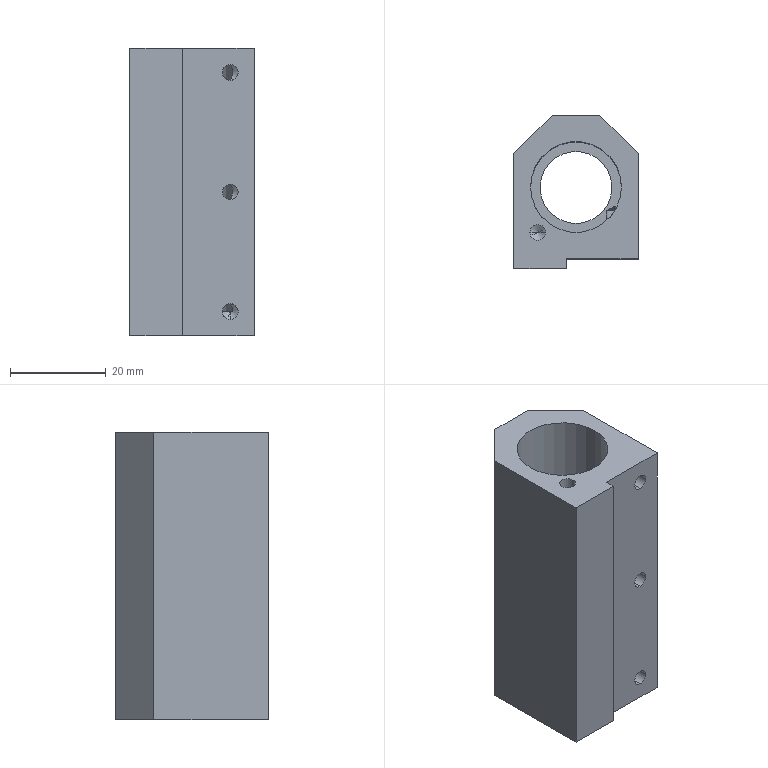Part | SolidWorks | features ICE 3, HoleWzd 2, 3DProfileFeature 1, Chamfer 1, Extrusion 1 | 1 solid | 29 faces | box 26 x 32 x 60 mm | volume 27463 mm3 | cylinder 12 | plane 11 | cone 6 | commonest cylinder face diameters 3.3 x8 15 x2 19 x2
STEP:
#1=CARTESIAN_POINT('',(-9.65,-9.5,49.9));
#2=VERTEX_POINT('',#1);
#3=CARTESIAN_POINT('',(-6.35,-9.5,49.9));
#4=VERTEX_POINT('',#3);
#5=CARTESIAN_POINT('',(-8.,-9.5,49.9));
#6=DIRECTION('',(0.,0.,1.));
#7=DIRECTION('',(1.,0.,0.));
#8=AXIS2_PLACEMENT_3D('',#5,#6,#7);
#9=CIRCLE('',#8,1.65);
#10=EDGE_CURVE('',#2,#4,#9,.T.);
#11=ORIENTED_EDGE('',*,*,#10,.F.);
#12=CARTESIAN_POINT('',(-9.65,-9.5,60.));
#13=VERTEX_POINT('',#12);
#14=CARTESIAN_POINT('',(-9.65,-9.5,60.));
#15=DIRECTION('',(0.,0.,1.));
#16=VECTOR('',#15,1000.);
#17=LINE('',#14,#16);
#18=EDGE_CURVE('',#2,#13,#17,.T.);
#19=ORIENTED_EDGE('',*,*,#18,.T.);
#20=CARTESIAN_POINT('',(-6.35,-9.5,60.));
#21=VERTEX_POINT('',#20);
#22=CARTESIAN_POINT('',(-8.,-9.5,60.));
#23=DIRECTION('',(0.,0.,1.));
#24=DIRECTION('',(1.,0.,0.));
#25=AXIS2_PLACEMENT_3D('',#22,#23,#24);
#26=CIRCLE('',#25,1.65);
#27=EDGE_CURVE('',#13,#21,#26,.T.);
#28=ORIENTED_EDGE('',*,*,#27,.T.);
#29=CARTESIAN_POINT('',(-6.35,-9.5,60.));
#30=DIRECTION('',(0.,0.,1.));
#31=VECTOR('',#30,1000.);
#32=LINE('',#29,#31);
#33=EDGE_CURVE('',#4,#21,#32,.T.);
#34=ORIENTED_EDGE('',*,*,#33,.F.);
#35=EDGE_LOOP('',(#11,#19,#28,#34));
#36=FACE_OUTER_BOUND('',#35,.T.);
#37=CARTESIAN_POINT('',(-8.,-9.5,60.));
#38=DIRECTION('',(0.,0.,1.));
#39=DIRECTION('',(1.,0.,0.));
#40=AXIS2_PLACEMENT_3D('',#37,#38,#39);
#41=CYLINDRICAL_SURFACE('',#40,1.65);
#42=ADVANCED_FACE('',(#36),#41,.F.);
#43=CARTESIAN_POINT('',(-8.,-9.5,48.909));
#44=VERTEX_POINT('',#43);
#45=CARTESIAN_POINT('',(-6.35,-9.5,49.9));
#46=DIRECTION('',(0.8572,0.,0.515));
#47=VECTOR('',#46,1000.);
#48=LINE('',#45,#47);
#49=EDGE_CURVE('',#44,#4,#48,.T.);
#50=ORIENTED_EDGE('',*,*,#49,.F.);
#51=CARTESIAN_POINT('',(-9.65,-9.5,49.9));
#52=DIRECTION('',(-0.8572,0.,0.515));
#53=VECTOR('',#52,1000.);
#54=LINE('',#51,#53);
#55=EDGE_CURVE('',#44,#2,#54,.T.);
#56=ORIENTED_EDGE('',*,*,#55,.T.);
#57=ORIENTED_EDGE('',*,*,#10,.T.);
#58=EDGE_LOOP('',(#50,#56,#57));
#59=FACE_OUTER_BOUND('',#58,.T.);
#60=CARTESIAN_POINT('',(-8.,-9.5,49.9));
#61=DIRECTION('',(0.,0.,1.));
#62=DIRECTION('',(1.,0.,0.));
#63=AXIS2_PLACEMENT_3D('',#60,#61,#62);
#64=CONICAL_SURFACE('',#63,1.65,1.03);
#65=ADVANCED_FACE('',(#59),#64,.F.);
#66=CARTESIAN_POINT('',(8.,-5.123,53.35));
#67=VERTEX_POINT('',#66);
#68=CARTESIAN_POINT('',(8.,-5.123,56.65));
#69=VERTEX_POINT('',#68);
#70=CARTESIAN_POINT('',(8.,-5.123,53.35));
#71=CARTESIAN_POINT('',(7.85,-5.358,53.35));
#72=CARTESIAN_POINT('',(7.69,-5.584,53.37));
#73=CARTESIAN_POINT('',(7.357,-6.017,53.471));
#74=CARTESIAN_POINT('',(7.179,-6.227,53.553));
#75=CARTESIAN_POINT('',(6.925,-6.504,53.743));
#76=CARTESIAN_POINT('',(6.841,-6.592,53.819));
#77=CARTESIAN_POINT('',(6.687,-6.749,53.994));
#78=CARTESIAN_POINT('',(6.616,-6.818,54.092));
#79=CARTESIAN_POINT('',(6.492,-6.936,54.317));
#80=CARTESIAN_POINT('',(6.441,-6.983,54.443));
#81=CARTESIAN_POINT('',(6.37,-7.048,54.708));
#82=CARTESIAN_POINT('',(6.351,-7.065,54.85));
#83=CARTESIAN_POINT('',(6.349,-7.067,55.132));
#84=CARTESIAN_POINT('',(6.367,-7.051,55.274));
#85=CARTESIAN_POINT('',(6.435,-6.988,55.541));
#86=CARTESIAN_POINT('',(6.486,-6.942,55.668));
#87=CARTESIAN_POINT('',(6.608,-6.826,55.895));
#88=CARTESIAN_POINT('',(6.68,-6.755,55.997));
#89=CARTESIAN_POINT('',(6.834,-6.599,56.174));
#90=CARTESIAN_POINT('',(6.918,-6.512,56.25));
#91=CARTESIAN_POINT('',(7.173,-6.234,56.443));
#92=CARTESIAN_POINT('',(7.348,-6.028,56.526));
#93=CARTESIAN_POINT('',(7.687,-5.589,56.63));
#94=CARTESIAN_POINT('',(7.848,-5.36,56.65));
#95=CARTESIAN_POINT('',(8.,-5.123,56.65));
#96=B_SPLINE_CURVE_WITH_KNOTS('',3,(#70,#71,#72,#73,#74,#75,#76,#77,#78,#79,#80,#81,#82,#83,#84,#85,#86,#87,#88,#89,#90,#91,#92,#93,#94,#95),.UNSPECIFIED.,.F.,.F.,(4,2,2,2,2,2,2,2,2,2,2,2,4),(0.0002601,0.00109,0.001921,0.002336,0.002751,0.003166,0.003582,0.003997,0.004412,0.004827,0.005242,0.006073,0.006903),.UNSPECIFIED.);
#97=EDGE_CURVE('',#67,#69,#96,.T.);
#98=ORIENTED_EDGE('',*,*,#97,.T.);
#99=CARTESIAN_POINT('',(8.,-15.,56.65));
#100=VERTEX_POINT('',#99);
#101=CARTESIAN_POINT('',(8.,-15.,56.65));
#102=DIRECTION('',(0.,-1.,0.));
#103=VECTOR('',#102,1000.);
#104=LINE('',#101,#103);
#105=EDGE_CURVE('',#69,#100,#104,.T.);
#106=ORIENTED_EDGE('',*,*,#105,.T.);
#107=CARTESIAN_POINT('',(8.,-15.,53.35));
#108=VERTEX_POINT('',#107);
#109=CARTESIAN_POINT('',(8.,-15.,55.));
#110=DIRECTION('',(0.,-1.,0.));
#111=DIRECTION('',(0.,0.,-1.));
#112=AXIS2_PLACEMENT_3D('',#109,#110,#111);
#113=CIRCLE('',#112,1.65);
#114=EDGE_CURVE('',#100,#108,#113,.T.);
#115=ORIENTED_EDGE('',*,*,#114,.T.);
#116=CARTESIAN_POINT('',(8.,-15.,53.35));
#117=DIRECTION('',(0.,-1.,0.));
#118=VECTOR('',#117,1000.);
#119=LINE('',#116,#118);
#120=EDGE_CURVE('',#67,#108,#119,.T.);
#121=ORIENTED_EDGE('',*,*,#120,.F.);
#122=EDGE_LOOP('',(#98,#106,#115,#121));
#123=FACE_OUTER_BOUND('',#122,.T.);
#124=CARTESIAN_POINT('',(8.,-15.,55.));
#125=DIRECTION('',(0.,-1.,0.));
#126=DIRECTION('',(0.,0.,-1.));
#127=AXIS2_PLACEMENT_3D('',#124,#125,#126);
#128=CYLINDRICAL_SURFACE('',#127,1.65);
#129=ADVANCED_FACE('',(#123),#128,.F.);
#130=CARTESIAN_POINT('',(8.,-5.123,28.35));
#131=VERTEX_POINT('',#130);
#132=CARTESIAN_POINT('',(8.,-5.123,31.65));
#133=VERTEX_POINT('',#132);
#134=CARTESIAN_POINT('',(8.,-5.123,28.35));
#135=CARTESIAN_POINT('',(7.85,-5.358,28.35));
#136=CARTESIAN_POINT('',(7.69,-5.584,28.37));
#137=CARTESIAN_POINT('',(7.357,-6.017,28.471));
#138=CARTESIAN_POINT('',(7.179,-6.227,28.553));
#139=CARTESIAN_POINT('',(6.925,-6.504,28.743));
#140=CARTESIAN_POINT('',(6.841,-6.592,28.819));
#141=CARTESIAN_POINT('',(6.687,-6.749,28.994));
#142=CARTESIAN_POINT('',(6.616,-6.818,29.092));
#143=CARTESIAN_POINT('',(6.492,-6.936,29.317));
#144=CARTESIAN_POINT('',(6.441,-6.983,29.443));
#145=CARTESIAN_POINT('',(6.37,-7.048,29.708));
#146=CARTESIAN_POINT('',(6.351,-7.065,29.85));
#147=CARTESIAN_POINT('',(6.349,-7.067,30.132));
#148=CARTESIAN_POINT('',(6.367,-7.051,30.274));
#149=CARTESIAN_POINT('',(6.435,-6.988,30.541));
#150=CARTESIAN_POINT('',(6.486,-6.942,30.668));
#151=CARTESIAN_POINT('',(6.608,-6.826,30.895));
#152=CARTESIAN_POINT('',(6.68,-6.755,30.997));
#153=CARTESIAN_POINT('',(6.834,-6.599,31.174));
#154=CARTESIAN_POINT('',(6.918,-6.512,31.25));
#155=CARTESIAN_POINT('',(7.173,-6.234,31.443));
#156=CARTESIAN_POINT('',(7.348,-6.028,31.526));
#157=CARTESIAN_POINT('',(7.687,-5.589,31.63));
#158=CARTESIAN_POINT('',(7.848,-5.36,31.65));
#159=CARTESIAN_POINT('',(8.,-5.123,31.65));
#160=B_SPLINE_CURVE_WITH_KNOTS('',3,(#134,#135,#136,#137,#138,#139,#140,#141,#142,#143,#144,#145,#146,#147,#148,#149,#150,#151,#152,#153,#154,#155,#156,#157,#158,#159),.UNSPECIFIED.,.F.,.F.,(4,2,2,2,2,2,2,2,2,2,2,2,4),(0.0002601,0.00109,0.001921,0.002336,0.002751,0.003166,0.003582,0.003997,0.004412,0.004827,0.005242,0.006073,0.006903),.UNSPECIFIED.);
#161=EDGE_CURVE('',#131,#133,#160,.T.);
#162=ORIENTED_EDGE('',*,*,#161,.T.);
#163=CARTESIAN_POINT('',(8.,-15.,31.65));
#164=VERTEX_POINT('',#163);
#165=CARTESIAN_POINT('',(8.,-15.,31.65));
#166=DIRECTION('',(0.,-1.,0.));
#167=VECTOR('',#166,1000.);
#168=LINE('',#165,#167);
#169=EDGE_CURVE('',#133,#164,#168,.T.);
#170=ORIENTED_EDGE('',*,*,#169,.T.);
#171=CARTESIAN_POINT('',(8.,-15.,28.35));
#172=VERTEX_POINT('',#171);
#173=CARTESIAN_POINT('',(8.,-15.,30.));
#174=DIRECTION('',(0.,-1.,0.));
#175=DIRECTION('',(0.,0.,-1.));
#176=AXIS2_PLACEMENT_3D('',#173,#174,#175);
#177=CIRCLE('',#176,1.65);
#178=EDGE_CURVE('',#164,#172,#177,.T.);
#179=ORIENTED_EDGE('',*,*,#178,.T.);
#180=CARTESIAN_POINT('',(8.,-15.,28.35));
#181=DIRECTION('',(0.,-1.,0.));
#182=VECTOR('',#181,1000.);
#183=LINE('',#180,#182);
#184=EDGE_CURVE('',#131,#172,#183,.T.);
#185=ORIENTED_EDGE('',*,*,#184,.F.);
#186=EDGE_LOOP('',(#162,#170,#179,#185));
#187=FACE_OUTER_BOUND('',#186,.T.);
#188=CARTESIAN_POINT('',(8.,-15.,30.));
#189=DIRECTION('',(0.,-1.,0.));
#190=DIRECTION('',(0.,0.,-1.));
#191=AXIS2_PLACEMENT_3D('',#188,#189,#190);
#192=CYLINDRICAL_SURFACE('',#191,1.65);
#193=ADVANCED_FACE('',(#187),#192,.F.);
#194=CARTESIAN_POINT('',(8.,-3.909,5.));
#195=VERTEX_POINT('',#194);
#196=CARTESIAN_POINT('',(8.513,-4.217,5.));
#197=VERTEX_POINT('',#196);
#198=CARTESIAN_POINT('',(8.,-3.909,5.));
#199=DIRECTION('',(0.8572,-0.515,0.));
#200=VECTOR('',#199,1000.);
#201=LINE('',#198,#200);
#202=EDGE_CURVE('',#195,#197,#201,.T.);
#203=ORIENTED_EDGE('',*,*,#202,.F.);
#204=CARTESIAN_POINT('',(8.,-4.9,3.35));
#205=VERTEX_POINT('',#204);
#206=CARTESIAN_POINT('',(8.,-4.9,3.35));
#207=DIRECTION('',(0.,-0.515,-0.8572));
#208=VECTOR('',#207,1000.);
#209=LINE('',#206,#208);
#210=EDGE_CURVE('',#195,#205,#209,.T.);
#211=ORIENTED_EDGE('',*,*,#210,.T.);
#212=CARTESIAN_POINT('',(8.139,-4.9,6.644));
#213=VERTEX_POINT('',#212);
#214=CARTESIAN_POINT('',(8.,-4.9,5.));
#215=DIRECTION('',(0.,-1.,0.));
#216=DIRECTION('',(0.,0.,-1.));
#217=AXIS2_PLACEMENT_3D('',#214,#215,#216);
#218=CIRCLE('',#217,1.65);
#219=EDGE_CURVE('',#205,#213,#218,.T.);
#220=ORIENTED_EDGE('',*,*,#219,.T.);
#221=CARTESIAN_POINT('',(8.139,-4.9,6.644));
#222=CARTESIAN_POINT('',(8.228,-4.752,6.39));
#223=CARTESIAN_POINT('',(8.31,-4.606,6.133));
#224=CARTESIAN_POINT('',(8.415,-4.41,5.729));
#225=CARTESIAN_POINT('',(8.447,-4.348,5.592));
#226=CARTESIAN_POINT('',(8.496,-4.251,5.305));
#227=CARTESIAN_POINT('',(8.513,-4.217,5.154));
#228=CARTESIAN_POINT('',(8.513,-4.217,5.));
#229=B_SPLINE_CURVE_WITH_KNOTS('',3,(#221,#222,#223,#224,#225,#226,#227,#228),.UNSPECIFIED.,.F.,.F.,(4,2,2,4),(0.0002054,0.001126,0.001587,0.002047),.UNSPECIFIED.);
#230=EDGE_CURVE('',#213,#197,#229,.T.);
#231=ORIENTED_EDGE('',*,*,#230,.T.);
#232=EDGE_LOOP('',(#203,#211,#220,#231));
#233=FACE_OUTER_BOUND('',#232,.T.);
#234=CARTESIAN_POINT('',(8.,-4.9,5.));
#235=DIRECTION('',(0.,-1.,0.));
#236=DIRECTION('',(0.,0.,-1.));
#237=AXIS2_PLACEMENT_3D('',#234,#235,#236);
#238=CONICAL_SURFACE('',#237,1.65,1.03);
#239=ADVANCED_FACE('',(#233),#238,.F.);
#240=CARTESIAN_POINT('',(6.35,-7.066,5.));
#241=VERTEX_POINT('',#240);
#242=CARTESIAN_POINT('',(8.,-5.123,6.65));
#243=VERTEX_POINT('',#242);
#244=CARTESIAN_POINT('',(6.35,-7.066,5.));
#245=CARTESIAN_POINT('',(6.35,-7.066,5.143));
#246=CARTESIAN_POINT('',(6.368,-7.05,5.281));
#247=CARTESIAN_POINT('',(6.438,-6.986,5.55));
#248=CARTESIAN_POINT('',(6.488,-6.94,5.674));
#249=CARTESIAN_POINT('',(6.673,-6.763,6.015));
#250=CARTESIAN_POINT('',(6.837,-6.6,6.19));
#251=CARTESIAN_POINT('',(7.091,-6.324,6.381));
#252=CARTESIAN_POINT('',(7.177,-6.226,6.433));
#253=CARTESIAN_POINT('',(7.349,-6.021,6.519));
#254=CARTESIAN_POINT('',(7.436,-5.914,6.553));
#255=CARTESIAN_POINT('',(7.689,-5.587,6.63));
#256=CARTESIAN_POINT('',(7.849,-5.359,6.65));
#257=CARTESIAN_POINT('',(8.,-5.123,6.65));
#258=B_SPLINE_CURVE_WITH_KNOTS('',3,(#244,#245,#246,#247,#248,#249,#250,#251,#252,#253,#254,#255,#256,#257),.UNSPECIFIED.,.F.,.F.,(4,2,2,2,2,2,4),(0.,0.0004216,0.0008433,0.001687,0.002108,0.00253,0.003373),.UNSPECIFIED.);
#259=EDGE_CURVE('',#241,#243,#258,.T.);
#260=ORIENTED_EDGE('',*,*,#259,.T.);
#261=CARTESIAN_POINT('',(8.,-15.,6.65));
#262=VERTEX_POINT('',#261);
#263=CARTESIAN_POINT('',(8.,-15.,6.65));
#264=DIRECTION('',(0.,-1.,0.));
#265=VECTOR('',#264,1000.);
#266=LINE('',#263,#265);
#267=EDGE_CURVE('',#243,#262,#266,.T.);
#268=ORIENTED_EDGE('',*,*,#267,.T.);
#269=CARTESIAN_POINT('',(8.,-15.,3.35));
#270=VERTEX_POINT('',#269);
#271=CARTESIAN_POINT('',(8.,-15.,5.));
#272=DIRECTION('',(0.,-1.,0.));
#273=DIRECTION('',(0.,0.,-1.));
#274=AXIS2_PLACEMENT_3D('',#271,#272,#273);
#275=CIRCLE('',#274,1.65);
#276=EDGE_CURVE('',#262,#270,#275,.T.);
#277=ORIENTED_EDGE('',*,*,#276,.T.);
#278=CARTESIAN_POINT('',(8.,-15.,3.35));
#279=DIRECTION('',(0.,-1.,0.));
#280=VECTOR('',#279,1000.);
#281=LINE('',#278,#280);
#282=EDGE_CURVE('',#205,#270,#281,.T.);
#283=ORIENTED_EDGE('',*,*,#282,.F.);
#284=CARTESIAN_POINT('',(6.35,-4.9,5.));
#285=VERTEX_POINT('',#284);
#286=CARTESIAN_POINT('',(8.,-4.9,5.));
#287=DIRECTION('',(0.,-1.,0.));
#288=DIRECTION('',(0.,0.,-1.));
#289=AXIS2_PLACEMENT_3D('',#286,#287,#288);
#290=CIRCLE('',#289,1.65);
#291=EDGE_CURVE('',#285,#205,#290,.T.);
#292=ORIENTED_EDGE('',*,*,#291,.F.);
#293=CARTESIAN_POINT('',(6.35,-15.,5.));
#294=DIRECTION('',(0.,1.,0.));
#295=VECTOR('',#294,1000.);
#296=LINE('',#293,#295);
#297=EDGE_CURVE('',#241,#285,#296,.T.);
#298=ORIENTED_EDGE('',*,*,#297,.F.);
#299=EDGE_LOOP('',(#260,#268,#277,#283,#292,#298));
#300=FACE_OUTER_BOUND('',#299,.T.);
#301=CARTESIAN_POINT('',(8.,-15.,5.));
#302=DIRECTION('',(0.,-1.,0.));
#303=DIRECTION('',(0.,0.,-1.));
#304=AXIS2_PLACEMENT_3D('',#301,#302,#303);
#305=CYLINDRICAL_SURFACE('',#304,1.65);
#306=ADVANCED_FACE('',(#300),#305,.F.);
#307=CARTESIAN_POINT('',(7.5,0.,5.));
#308=VERTEX_POINT('',#307);
#309=CARTESIAN_POINT('',(-7.5,0.,5.));
#310=VERTEX_POINT('',#309);
#311=CARTESIAN_POINT('',(0.,0.,5.));
#312=DIRECTION('',(0.,0.,-1.));
#313=DIRECTION('',(-1.,0.,0.));
#314=AXIS2_PLACEMENT_3D('',#311,#312,#313);
#315=CIRCLE('',#314,7.5);
#316=EDGE_CURVE('',#308,#310,#315,.T.);
#317=ORIENTED_EDGE('',*,*,#316,.F.);
#318=CARTESIAN_POINT('',(7.5,0.,0.));
#319=VERTEX_POINT('',#318);
#320=CARTESIAN_POINT('',(7.5,0.,5.));
#321=DIRECTION('',(0.,0.,-1.));
#322=VECTOR('',#321,1000.);
#323=LINE('',#320,#322);
#324=EDGE_CURVE('',#308,#319,#323,.T.);
#325=ORIENTED_EDGE('',*,*,#324,.T.);
#326=CARTESIAN_POINT('',(-7.5,0.,0.));
#327=VERTEX_POINT('',#326);
#328=CARTESIAN_POINT('',(0.,0.,0.));
#329=DIRECTION('',(0.,0.,-1.));
#330=DIRECTION('',(-1.,0.,0.));
#331=AXIS2_PLACEMENT_3D('',#328,#329,#330);
#332=CIRCLE('',#331,7.5);
#333=EDGE_CURVE('',#319,#327,#332,.T.);
#334=ORIENTED_EDGE('',*,*,#333,.T.);
#335=CARTESIAN_POINT('',(-7.5,0.,5.));
#336=DIRECTION('',(0.,0.,-1.));
#337=VECTOR('',#336,1000.);
#338=LINE('',#335,#337);
#339=EDGE_CURVE('',#310,#327,#338,.T.);
#340=ORIENTED_EDGE('',*,*,#339,.F.);
#341=EDGE_LOOP('',(#317,#325,#334,#340));
#342=FACE_OUTER_BOUND('',#341,.T.);
#343=CARTESIAN_POINT('',(0.,0.,5.));
#344=DIRECTION('',(0.,0.,-1.));
#345=DIRECTION('',(-1.,0.,0.));
#346=AXIS2_PLACEMENT_3D('',#343,#344,#345);
#347=CYLINDRICAL_SURFACE('',#346,7.5);
#348=ADVANCED_FACE('',(#342),#347,.F.);
#349=CARTESIAN_POINT('',(8.139,-4.9,53.356));
#350=VERTEX_POINT('',#349);
#351=CARTESIAN_POINT('',(8.139,-4.9,53.356));
#352=CARTESIAN_POINT('',(8.093,-4.975,53.352));
#353=CARTESIAN_POINT('',(8.047,-5.05,53.35));
#354=CARTESIAN_POINT('',(8.,-5.123,53.35));
#355=B_SPLINE_CURVE_WITH_KNOTS('',3,(#351,#352,#353,#354),.UNSPECIFIED.,.F.,.F.,(4,4),(0.,0.0002601),.UNSPECIFIED.);
#356=EDGE_CURVE('',#350,#67,#355,.T.);
#357=ORIENTED_EDGE('',*,*,#356,.F.);
#358=CARTESIAN_POINT('',(8.139,-4.9,56.644));
#359=VERTEX_POINT('',#358);
#360=CARTESIAN_POINT('',(8.139,-4.9,56.644));
#361=CARTESIAN_POINT('',(8.228,-4.752,56.389));
#362=CARTESIAN_POINT('',(8.31,-4.606,56.131));
#363=CARTESIAN_POINT('',(8.415,-4.409,55.726));
#364=CARTESIAN_POINT('',(8.447,-4.347,55.589));
#365=CARTESIAN_POINT('',(8.497,-4.25,55.301));
#366=CARTESIAN_POINT('',(8.513,-4.216,55.15));
#367=CARTESIAN_POINT('',(8.513,-4.217,54.84));
#368=CARTESIAN_POINT('',(8.495,-4.252,54.689));
#369=CARTESIAN_POINT('',(8.445,-4.351,54.402));
#370=CARTESIAN_POINT('',(8.414,-4.412,54.266));
#371=CARTESIAN_POINT('',(8.309,-4.608,53.866));
#372=CARTESIAN_POINT('',(8.227,-4.753,53.609));
#373=CARTESIAN_POINT('',(8.139,-4.9,53.356));
#374=B_SPLINE_CURVE_WITH_KNOTS('',3,(#360,#361,#362,#363,#364,#365,#366,#367,#368,#369,#370,#371,#372,#373),.UNSPECIFIED.,.F.,.F.,(4,2,2,2,2,2,4),(0.0002054,0.001129,0.00159,0.002052,0.002514,0.002975,0.003899),.UNSPECIFIED.);
#375=EDGE_CURVE('',#359,#350,#374,.T.);
#376=ORIENTED_EDGE('',*,*,#375,.F.);
#377=CARTESIAN_POINT('',(8.,-5.123,56.65));
#378=CARTESIAN_POINT('',(8.047,-5.05,56.65));
#379=CARTESIAN_POINT('',(8.093,-4.975,56.648));
#380=CARTESIAN_POINT('',(8.139,-4.9,56.644));
#381=B_SPLINE_CURVE_WITH_KNOTS('',3,(#377,#378,#379,#380),.UNSPECIFIED.,.F.,.F.,(4,4),(0.006903,0.007161),.UNSPECIFIED.);
#382=EDGE_CURVE('',#69,#359,#381,.T.);
#383=ORIENTED_EDGE('',*,*,#382,.F.);
#384=ORIENTED_EDGE('',*,*,#97,.F.);
#385=EDGE_LOOP('',(#357,#376,#383,#384));
#386=FACE_BOUND('',#385,.T.);
#387=CARTESIAN_POINT('',(8.139,-4.9,28.356));
#388=VERTEX_POINT('',#387);
#389=CARTESIAN_POINT('',(8.139,-4.9,28.356));
#390=CARTESIAN_POINT('',(8.093,-4.975,28.352));
#391=CARTESIAN_POINT('',(8.047,-5.05,28.35));
#392=CARTESIAN_POINT('',(8.,-5.123,28.35));
#393=B_SPLINE_CURVE_WITH_KNOTS('',3,(#389,#390,#391,#392),.UNSPECIFIED.,.F.,.F.,(4,4),(0.,0.0002601),.UNSPECIFIED.);
#394=EDGE_CURVE('',#388,#131,#393,.T.);
#395=ORIENTED_EDGE('',*,*,#394,.F.);
#396=CARTESIAN_POINT('',(8.139,-4.9,31.644));
#397=VERTEX_POINT('',#396);
#398=CARTESIAN_POINT('',(8.139,-4.9,31.644));
#399=CARTESIAN_POINT('',(8.228,-4.752,31.389));
#400=CARTESIAN_POINT('',(8.31,-4.606,31.131));
#401=CARTESIAN_POINT('',(8.415,-4.409,30.726));
#402=CARTESIAN_POINT('',(8.447,-4.347,30.589));
#403=CARTESIAN_POINT('',(8.497,-4.25,30.301));
#404=CARTESIAN_POINT('',(8.513,-4.216,30.15));
#405=CARTESIAN_POINT('',(8.513,-4.217,29.84));
#406=CARTESIAN_POINT('',(8.495,-4.252,29.689));
#407=CARTESIAN_POINT('',(8.445,-4.351,29.402));
#408=CARTESIAN_POINT('',(8.414,-4.412,29.266));
#409=CARTESIAN_POINT('',(8.309,-4.608,28.866));
#410=CARTESIAN_POINT('',(8.227,-4.753,28.609));
#411=CARTESIAN_POINT('',(8.139,-4.9,28.356));
#412=B_SPLINE_CURVE_WITH_KNOTS('',3,(#398,#399,#400,#401,#402,#403,#404,#405,#406,#407,#408,#409,#410,#411),.UNSPECIFIED.,.F.,.F.,(4,2,2,2,2,2,4),(0.0002054,0.001129,0.00159,0.002052,0.002514,0.002975,0.003899),.UNSPECIFIED.);
#413=EDGE_CURVE('',#397,#388,#412,.T.);
#414=ORIENTED_EDGE('',*,*,#413,.F.);
#415=CARTESIAN_POINT('',(8.,-5.123,31.65));
#416=CARTESIAN_POINT('',(8.047,-5.05,31.65));
#417=CARTESIAN_POINT('',(8.093,-4.975,31.648));
#418=CARTESIAN_POINT('',(8.139,-4.9,31.644));
#419=B_SPLINE_CURVE_WITH_KNOTS('',3,(#415,#416,#417,#418),.UNSPECIFIED.,.F.,.F.,(4,4),(0.006903,0.007161),.UNSPECIFIED.);
#420=EDGE_CURVE('',#133,#397,#419,.T.);
#421=ORIENTED_EDGE('',*,*,#420,.F.);
#422=ORIENTED_EDGE('',*,*,#161,.F.);
#423=EDGE_LOOP('',(#395,#414,#421,#422));
#424=FACE_BOUND('',#423,.T.);
#425=CARTESIAN_POINT('',(-9.5,0.,60.));
#426=VERTEX_POINT('',#425);
#427=CARTESIAN_POINT('',(9.5,0.,60.));
#428=VERTEX_POINT('',#427);
#429=CARTESIAN_POINT('',(0.,0.,60.));
#430=DIRECTION('',(0.,0.,1.));
#431=DIRECTION('',(1.,0.,0.));
#432=AXIS2_PLACEMENT_3D('',#429,#430,#431);
#433=CIRCLE('',#432,9.5);
#434=EDGE_CURVE('',#426,#428,#433,.T.);
#435=ORIENTED_EDGE('',*,*,#434,.T.);
#436=CARTESIAN_POINT('',(9.5,0.,5.));
#437=VERTEX_POINT('',#436);
#438=CARTESIAN_POINT('',(9.5,0.,60.));
#439=DIRECTION('',(0.,0.,-1.));
#440=VECTOR('',#439,1000.);
#441=LINE('',#438,#440);
#442=EDGE_CURVE('',#428,#437,#441,.T.);
#443=ORIENTED_EDGE('',*,*,#442,.T.);
#444=CARTESIAN_POINT('',(0.,0.,5.));
#445=DIRECTION('',(0.,0.,-1.));
#446=DIRECTION('',(-1.,0.,0.));
#447=AXIS2_PLACEMENT_3D('',#444,#445,#446);
#448=CIRCLE('',#447,9.5);
#449=EDGE_CURVE('',#437,#197,#448,.T.);
#450=ORIENTED_EDGE('',*,*,#449,.T.);
#451=ORIENTED_EDGE('',*,*,#230,.F.);
#452=CARTESIAN_POINT('',(8.,-5.123,6.65));
#453=CARTESIAN_POINT('',(8.047,-5.05,6.65));
#454=CARTESIAN_POINT('',(8.093,-4.975,6.648));
#455=CARTESIAN_POINT('',(8.139,-4.9,6.644));
#456=B_SPLINE_CURVE_WITH_KNOTS('',3,(#452,#453,#454,#455),.UNSPECIFIED.,.F.,.F.,(4,4),(0.003373,0.003636),.UNSPECIFIED.);
#457=EDGE_CURVE('',#243,#213,#456,.T.);
#458=ORIENTED_EDGE('',*,*,#457,.F.);
#459=ORIENTED_EDGE('',*,*,#259,.F.);
#460=CARTESIAN_POINT('',(-9.5,0.,5.));
#461=VERTEX_POINT('',#460);
#462=CARTESIAN_POINT('',(0.,0.,5.));
#463=DIRECTION('',(0.,0.,-1.));
#464=DIRECTION('',(-1.,0.,0.));
#465=AXIS2_PLACEMENT_3D('',#462,#463,#464);
#466=CIRCLE('',#465,9.5);
#467=EDGE_CURVE('',#241,#461,#466,.T.);
#468=ORIENTED_EDGE('',*,*,#467,.T.);
#469=CARTESIAN_POINT('',(-9.5,0.,60.));
#470=DIRECTION('',(0.,0.,-1.));
#471=VECTOR('',#470,1000.);
#472=LINE('',#469,#471);
#473=EDGE_CURVE('',#426,#461,#472,.T.);
#474=ORIENTED_EDGE('',*,*,#473,.F.);
#475=EDGE_LOOP('',(#435,#443,#450,#451,#458,#459,#468,#474));
#476=FACE_OUTER_BOUND('',#475,.T.);
#477=CARTESIAN_POINT('',(0.,0.,60.));
#478=DIRECTION('',(0.,0.,-1.));
#479=DIRECTION('',(-1.,0.,0.));
#480=AXIS2_PLACEMENT_3D('',#477,#478,#479);
#481=CYLINDRICAL_SURFACE('',#480,9.5);
#482=ADVANCED_FACE('',(#386,#424,#476),#481,.F.);
#483=CARTESIAN_POINT('',(8.,-15.,55.));
#484=DIRECTION('',(0.,-1.,0.));
#485=DIRECTION('',(0.,0.,-1.));
#486=AXIS2_PLACEMENT_3D('',#483,#484,#485);
#487=CIRCLE('',#486,1.65);
#488=EDGE_CURVE('',#108,#100,#487,.T.);
#489=ORIENTED_EDGE('',*,*,#488,.F.);
#490=ORIENTED_EDGE('',*,*,#114,.F.);
#491=EDGE_LOOP('',(#489,#490));
#492=FACE_BOUND('',#491,.T.);
#493=CARTESIAN_POINT('',(8.,-15.,30.));
#494=DIRECTION('',(0.,-1.,0.));
#495=DIRECTION('',(0.,0.,-1.));
#496=AXIS2_PLACEMENT_3D('',#493,#494,#495);
#497=CIRCLE('',#496,1.65);
#498=EDGE_CURVE('',#172,#164,#497,.T.);
#499=ORIENTED_EDGE('',*,*,#498,.F.);
#500=ORIENTED_EDGE('',*,*,#178,.F.);
#501=EDGE_LOOP('',(#499,#500));
#502=FACE_BOUND('',#501,.T.);
#503=CARTESIAN_POINT('',(8.,-15.,5.));
#504=DIRECTION('',(0.,-1.,0.));
#505=DIRECTION('',(0.,0.,-1.));
#506=AXIS2_PLACEMENT_3D('',#503,#504,#505);
#507=CIRCLE('',#506,1.65);
#508=EDGE_CURVE('',#270,#262,#507,.T.);
#509=ORIENTED_EDGE('',*,*,#508,.F.);
#510=ORIENTED_EDGE('',*,*,#276,.F.);
#511=EDGE_LOOP('',(#509,#510));
#512=FACE_BOUND('',#511,.T.);
#513=CARTESIAN_POINT('',(-2.,-15.,0.));
#514=VERTEX_POINT('',#513);
#515=CARTESIAN_POINT('',(-2.,-15.,60.));
#516=VERTEX_POINT('',#515);
#517=CARTESIAN_POINT('',(-2.,-15.,60.));
#518=DIRECTION('',(0.,0.,1.));
#519=VECTOR('',#518,1000.);
#520=LINE('',#517,#519);
#521=EDGE_CURVE('',#514,#516,#520,.T.);
#522=ORIENTED_EDGE('',*,*,#521,.F.);
#523=CARTESIAN_POINT('',(13.,-15.,0.));
#524=VERTEX_POINT('',#523);
#525=CARTESIAN_POINT('',(-13.,-15.,0.));
#526=DIRECTION('',(1.,0.,0.));
#527=VECTOR('',#526,1000.);
#528=LINE('',#525,#527);
#529=EDGE_CURVE('',#514,#524,#528,.T.);
#530=ORIENTED_EDGE('',*,*,#529,.T.);
#531=CARTESIAN_POINT('',(13.,-15.,60.));
#532=VERTEX_POINT('',#531);
#533=CARTESIAN_POINT('',(13.,-15.,60.));
#534=DIRECTION('',(0.,0.,-1.));
#535=VECTOR('',#534,1000.);
#536=LINE('',#533,#535);
#537=EDGE_CURVE('',#532,#524,#536,.T.);
#538=ORIENTED_EDGE('',*,*,#537,.F.);
#539=CARTESIAN_POINT('',(-13.,-15.,60.));
#540=DIRECTION('',(1.,0.,0.));
#541=VECTOR('',#540,1000.);
#542=LINE('',#539,#541);
#543=EDGE_CURVE('',#516,#532,#542,.T.);
#544=ORIENTED_EDGE('',*,*,#543,.F.);
#545=EDGE_LOOP('',(#522,#530,#538,#544));
#546=FACE_OUTER_BOUND('',#545,.T.);
#547=CARTESIAN_POINT('',(-13.,-15.,60.));
#548=DIRECTION('',(0.,1.,0.));
#549=DIRECTION('',(0.,0.,1.));
#550=AXIS2_PLACEMENT_3D('',#547,#548,#549);
#551=PLANE('',#550);
#552=ADVANCED_FACE('',(#492,#502,#512,#546),#551,.F.);
#553=ORIENTED_EDGE('',*,*,#442,.F.);
#554=CARTESIAN_POINT('',(0.,0.,60.));
#555=DIRECTION('',(0.,0.,1.));
#556=DIRECTION('',(1.,0.,0.));
#557=AXIS2_PLACEMENT_3D('',#554,#555,#556);
#558=CIRCLE('',#557,9.5);
#559=EDGE_CURVE('',#428,#426,#558,.T.);
#560=ORIENTED_EDGE('',*,*,#559,.T.);
#561=ORIENTED_EDGE('',*,*,#473,.T.);
#562=CARTESIAN_POINT('',(0.,0.,5.));
#563=DIRECTION('',(0.,0.,-1.));
#564=DIRECTION('',(-1.,0.,0.));
#565=AXIS2_PLACEMENT_3D('',#562,#563,#564);
#566=CIRCLE('',#565,9.5);
#567=EDGE_CURVE('',#461,#437,#566,.T.);
#568=ORIENTED_EDGE('',*,*,#567,.T.);
#569=EDGE_LOOP('',(#553,#560,#561,#568));
#570=FACE_OUTER_BOUND('',#569,.T.);
#571=CARTESIAN_POINT('',(0.,0.,60.));
#572=DIRECTION('',(0.,0.,-1.));
#573=DIRECTION('',(-1.,0.,0.));
#574=AXIS2_PLACEMENT_3D('',#571,#572,#573);
#575=CYLINDRICAL_SURFACE('',#574,9.5);
#576=ADVANCED_FACE('',(#570),#575,.F.);
#577=CARTESIAN_POINT('',(-8.,-9.5,60.));
#578=DIRECTION('',(0.,0.,1.));
#579=DIRECTION('',(1.,0.,0.));
#580=AXIS2_PLACEMENT_3D('',#577,#578,#579);
#581=CIRCLE('',#580,1.65);
#582=EDGE_CURVE('',#21,#13,#581,.T.);
#583=ORIENTED_EDGE('',*,*,#582,.F.);
#584=ORIENTED_EDGE('',*,*,#27,.F.);
#585=EDGE_LOOP('',(#583,#584));
#586=FACE_BOUND('',#585,.T.);
#587=CARTESIAN_POINT('',(13.,7.,60.));
#588=VERTEX_POINT('',#587);
#589=CARTESIAN_POINT('',(13.,15.,60.));
#590=DIRECTION('',(0.,1.,0.));
#591=VECTOR('',#590,1000.);
#592=LINE('',#589,#591);
#593=EDGE_CURVE('',#532,#588,#592,.T.);
#594=ORIENTED_EDGE('',*,*,#593,.T.);
#595=CARTESIAN_POINT('',(5.,15.,60.));
#596=VERTEX_POINT('',#595);
#597=CARTESIAN_POINT('',(10.,10.,60.));
#598=DIRECTION('',(-0.7071,0.7071,0.));
#599=VECTOR('',#598,1000.);
#600=LINE('',#597,#599);
#601=EDGE_CURVE('',#588,#596,#600,.T.);
#602=ORIENTED_EDGE('',*,*,#601,.T.);
#603=CARTESIAN_POINT('',(-5.,15.,60.));
#604=VERTEX_POINT('',#603);
#605=CARTESIAN_POINT('',(-13.,15.,60.));
#606=DIRECTION('',(-1.,0.,0.));
#607=VECTOR('',#606,1000.);
#608=LINE('',#605,#607);
#609=EDGE_CURVE('',#596,#604,#608,.T.);
#610=ORIENTED_EDGE('',*,*,#609,.T.);
#611=CARTESIAN_POINT('',(-13.,7.,60.));
#612=VERTEX_POINT('',#611);
#613=CARTESIAN_POINT('',(-10.,10.,60.));
#614=DIRECTION('',(-0.7071,-0.7071,0.));
#615=VECTOR('',#614,1000.);
#616=LINE('',#613,#615);
#617=EDGE_CURVE('',#604,#612,#616,.T.);
#618=ORIENTED_EDGE('',*,*,#617,.T.);
#619=CARTESIAN_POINT('',(-13.,-17.,60.));
#620=VERTEX_POINT('',#619);
#621=CARTESIAN_POINT('',(-13.,15.,60.));
#622=DIRECTION('',(0.,-1.,0.));
#623=VECTOR('',#622,1000.);
#624=LINE('',#621,#623);
#625=EDGE_CURVE('',#612,#620,#624,.T.);
#626=ORIENTED_EDGE('',*,*,#625,.T.);
#627=CARTESIAN_POINT('',(-2.,-17.,60.));
#628=VERTEX_POINT('',#627);
#629=CARTESIAN_POINT('',(-13.,-17.,60.));
#630=DIRECTION('',(-1.,0.,0.));
#631=VECTOR('',#630,1000.);
#632=LINE('',#629,#631);
#633=EDGE_CURVE('',#628,#620,#632,.T.);
#634=ORIENTED_EDGE('',*,*,#633,.F.);
#635=CARTESIAN_POINT('',(-2.,-17.,60.));
#636=DIRECTION('',(0.,1.,0.));
#637=VECTOR('',#636,1000.);
#638=LINE('',#635,#637);
#639=EDGE_CURVE('',#628,#516,#638,.T.);
#640=ORIENTED_EDGE('',*,*,#639,.T.);
#641=ORIENTED_EDGE('',*,*,#543,.T.);
#642=EDGE_LOOP('',(#594,#602,#610,#618,#626,#634,#640,#641));
#643=FACE_OUTER_BOUND('',#642,.T.);
#644=ORIENTED_EDGE('',*,*,#434,.F.);
#645=ORIENTED_EDGE('',*,*,#559,.F.);
#646=EDGE_LOOP('',(#644,#645));
#647=FACE_BOUND('',#646,.T.);
#648=CARTESIAN_POINT('',(0.,0.,60.));
#649=DIRECTION('',(0.,0.,1.));
#650=DIRECTION('',(1.,0.,0.));
#651=AXIS2_PLACEMENT_3D('',#648,#649,#650);
#652=PLANE('',#651);
#653=ADVANCED_FACE('',(#586,#643,#647),#652,.T.);
#654=CARTESIAN_POINT('',(5.,15.,0.));
#655=VERTEX_POINT('',#654);
#656=CARTESIAN_POINT('',(-5.,15.,0.));
#657=VERTEX_POINT('',#656);
#658=CARTESIAN_POINT('',(-13.,15.,0.));
#659=DIRECTION('',(-1.,0.,0.));
#660=VECTOR('',#659,1000.);
#661=LINE('',#658,#660);
#662=EDGE_CURVE('',#655,#657,#661,.T.);
#663=ORIENTED_EDGE('',*,*,#662,.F.);
#664=CARTESIAN_POINT('',(13.,7.,0.));
#665=VERTEX_POINT('',#664);
#666=CARTESIAN_POINT('',(5.,15.,0.));
#667=DIRECTION('',(0.7071,-0.7071,0.));
#668=VECTOR('',#667,1000.);
#669=LINE('',#666,#668);
#670=EDGE_CURVE('',#655,#665,#669,.T.);
#671=ORIENTED_EDGE('',*,*,#670,.T.);
#672=CARTESIAN_POINT('',(13.,15.,0.));
#673=DIRECTION('',(0.,1.,0.));
#674=VECTOR('',#673,1000.);
#675=LINE('',#672,#674);
#676=EDGE_CURVE('',#524,#665,#675,.T.);
#677=ORIENTED_EDGE('',*,*,#676,.F.);
#678=ORIENTED_EDGE('',*,*,#529,.F.);
#679=CARTESIAN_POINT('',(-2.,-17.,0.));
#680=VERTEX_POINT('',#679);
#681=CARTESIAN_POINT('',(-2.,-17.,0.));
#682=DIRECTION('',(0.,1.,0.));
#683=VECTOR('',#682,1000.);
#684=LINE('',#681,#683);
#685=EDGE_CURVE('',#680,#514,#684,.T.);
#686=ORIENTED_EDGE('',*,*,#685,.F.);
#687=CARTESIAN_POINT('',(-13.,-17.,0.));
#688=VERTEX_POINT('',#687);
#689=CARTESIAN_POINT('',(-13.,-17.,0.));
#690=DIRECTION('',(1.,0.,0.));
#691=VECTOR('',#690,1000.);
#692=LINE('',#689,#691);
#693=EDGE_CURVE('',#688,#680,#692,.T.);
#694=ORIENTED_EDGE('',*,*,#693,.F.);
#695=CARTESIAN_POINT('',(-13.,7.,0.));
#696=VERTEX_POINT('',#695);
#697=CARTESIAN_POINT('',(-13.,15.,0.));
#698=DIRECTION('',(0.,-1.,0.));
#699=VECTOR('',#698,1000.);
#700=LINE('',#697,#699);
#701=EDGE_CURVE('',#696,#688,#700,.T.);
#702=ORIENTED_EDGE('',*,*,#701,.F.);
#703=CARTESIAN_POINT('',(-13.,7.,0.));
#704=DIRECTION('',(0.7071,0.7071,0.));
#705=VECTOR('',#704,1000.);
#706=LINE('',#703,#705);
#707=EDGE_CURVE('',#696,#657,#706,.T.);
#708=ORIENTED_EDGE('',*,*,#707,.T.);
#709=EDGE_LOOP('',(#663,#671,#677,#678,#686,#694,#702,#708));
#710=FACE_OUTER_BOUND('',#709,.T.);
#711=CARTESIAN_POINT('',(0.,0.,0.));
#712=DIRECTION('',(0.,0.,-1.));
#713=DIRECTION('',(-1.,0.,0.));
#714=AXIS2_PLACEMENT_3D('',#711,#712,#713);
#715=CIRCLE('',#714,7.5);
#716=EDGE_CURVE('',#327,#319,#715,.T.);
#717=ORIENTED_EDGE('',*,*,#716,.F.);
#718=ORIENTED_EDGE('',*,*,#333,.F.);
#719=EDGE_LOOP('',(#717,#718));
#720=FACE_BOUND('',#719,.T.);
#721=CARTESIAN_POINT('',(0.,0.,0.));
#722=DIRECTION('',(0.,0.,1.));
#723=DIRECTION('',(1.,0.,0.));
#724=AXIS2_PLACEMENT_3D('',#721,#722,#723);
#725=PLANE('',#724);
#726=ADVANCED_FACE('',(#710,#720),#725,.F.);
#727=ORIENTED_EDGE('',*,*,#676,.T.);
#728=CARTESIAN_POINT('',(13.,7.,60.));
#729=DIRECTION('',(0.,0.,1.));
#730=VECTOR('',#729,1000.);
#731=LINE('',#728,#730);
#732=EDGE_CURVE('',#665,#588,#731,.T.);
#733=ORIENTED_EDGE('',*,*,#732,.T.);
#734=ORIENTED_EDGE('',*,*,#593,.F.);
#735=ORIENTED_EDGE('',*,*,#537,.T.);
#736=EDGE_LOOP('',(#727,#733,#734,#735));
#737=FACE_OUTER_BOUND('',#736,.T.);
#738=CARTESIAN_POINT('',(13.,15.,60.));
#739=DIRECTION('',(-1.,0.,0.));
#740=DIRECTION('',(0.,-1.,0.));
#741=AXIS2_PLACEMENT_3D('',#738,#739,#740);
#742=PLANE('',#741);
#743=ADVANCED_FACE('',(#737),#742,.F.);
#744=ORIENTED_EDGE('',*,*,#609,.F.);
#745=CARTESIAN_POINT('',(5.,15.,60.));
#746=DIRECTION('',(0.,0.,-1.));
#747=VECTOR('',#746,1000.);
#748=LINE('',#745,#747);
#749=EDGE_CURVE('',#596,#655,#748,.T.);
#750=ORIENTED_EDGE('',*,*,#749,.T.);
#751=ORIENTED_EDGE('',*,*,#662,.T.);
#752=CARTESIAN_POINT('',(-5.,15.,60.));
#753=DIRECTION('',(0.,0.,1.));
#754=VECTOR('',#753,1000.);
#755=LINE('',#752,#754);
#756=EDGE_CURVE('',#657,#604,#755,.T.);
#757=ORIENTED_EDGE('',*,*,#756,.T.);
#758=EDGE_LOOP('',(#744,#750,#751,#757));
#759=FACE_OUTER_BOUND('',#758,.T.);
#760=CARTESIAN_POINT('',(-13.,15.,60.));
#761=DIRECTION('',(0.,-1.,0.));
#762=DIRECTION('',(0.,0.,-1.));
#763=AXIS2_PLACEMENT_3D('',#760,#761,#762);
#764=PLANE('',#763);
#765=ADVANCED_FACE('',(#759),#764,.F.);
#766=ORIENTED_EDGE('',*,*,#625,.F.);
#767=CARTESIAN_POINT('',(-13.,7.,60.));
#768=DIRECTION('',(0.,0.,-1.));
#769=VECTOR('',#768,1000.);
#770=LINE('',#767,#769);
#771=EDGE_CURVE('',#612,#696,#770,.T.);
#772=ORIENTED_EDGE('',*,*,#771,.T.);
#773=ORIENTED_EDGE('',*,*,#701,.T.);
#774=CARTESIAN_POINT('',(-13.,-17.,60.));
#775=DIRECTION('',(0.,0.,-1.));
#776=VECTOR('',#775,1000.);
#777=LINE('',#774,#776);
#778=EDGE_CURVE('',#620,#688,#777,.T.);
#779=ORIENTED_EDGE('',*,*,#778,.F.);
#780=EDGE_LOOP('',(#766,#772,#773,#779));
#781=FACE_OUTER_BOUND('',#780,.T.);
#782=CARTESIAN_POINT('',(-13.,15.,60.));
#783=DIRECTION('',(1.,0.,0.));
#784=DIRECTION('',(0.,1.,0.));
#785=AXIS2_PLACEMENT_3D('',#782,#783,#784);
#786=PLANE('',#785);
#787=ADVANCED_FACE('',(#781),#786,.F.);
#788=CARTESIAN_POINT('',(0.,0.,5.));
#789=DIRECTION('',(0.,0.,-1.));
#790=DIRECTION('',(-1.,0.,0.));
#791=AXIS2_PLACEMENT_3D('',#788,#789,#790);
#792=CIRCLE('',#791,7.5);
#793=EDGE_CURVE('',#310,#308,#792,.T.);
#794=ORIENTED_EDGE('',*,*,#793,.T.);
#795=ORIENTED_EDGE('',*,*,#316,.T.);
#796=EDGE_LOOP('',(#794,#795));
#797=FACE_BOUND('',#796,.T.);
#798=CARTESIAN_POINT('',(8.,-3.909,5.));
#799=DIRECTION('',(0.8572,0.515,0.));
#800=VECTOR('',#799,1000.);
#801=LINE('',#798,#800);
#802=EDGE_CURVE('',#285,#195,#801,.T.);
#803=ORIENTED_EDGE('',*,*,#802,.T.);
#804=ORIENTED_EDGE('',*,*,#202,.T.);
#805=ORIENTED_EDGE('',*,*,#449,.F.);
#806=ORIENTED_EDGE('',*,*,#567,.F.);
#807=ORIENTED_EDGE('',*,*,#467,.F.);
#808=ORIENTED_EDGE('',*,*,#297,.T.);
#809=EDGE_LOOP('',(#803,#804,#805,#806,#807,#808));
#810=FACE_OUTER_BOUND('',#809,.T.);
#811=CARTESIAN_POINT('',(0.,0.,5.));
#812=DIRECTION('',(0.,0.,-1.));
#813=DIRECTION('',(-1.,0.,0.));
#814=AXIS2_PLACEMENT_3D('',#811,#812,#813);
#815=PLANE('',#814);
#816=ADVANCED_FACE('',(#797,#810),#815,.F.);
#817=ORIENTED_EDGE('',*,*,#324,.F.);
#818=ORIENTED_EDGE('',*,*,#793,.F.);
#819=ORIENTED_EDGE('',*,*,#339,.T.);
#820=ORIENTED_EDGE('',*,*,#716,.T.);
#821=EDGE_LOOP('',(#817,#818,#819,#820));
#822=FACE_OUTER_BOUND('',#821,.T.);
#823=CARTESIAN_POINT('',(0.,0.,5.));
#824=DIRECTION('',(0.,0.,-1.));
#825=DIRECTION('',(-1.,0.,0.));
#826=AXIS2_PLACEMENT_3D('',#823,#824,#825);
#827=CYLINDRICAL_SURFACE('',#826,7.5);
#828=ADVANCED_FACE('',(#822),#827,.F.);
#829=ORIENTED_EDGE('',*,*,#521,.T.);
#830=ORIENTED_EDGE('',*,*,#639,.F.);
#831=CARTESIAN_POINT('',(-2.,-17.,60.));
#832=DIRECTION('',(0.,0.,1.));
#833=VECTOR('',#832,1000.);
#834=LINE('',#831,#833);
#835=EDGE_CURVE('',#680,#628,#834,.T.);
#836=ORIENTED_EDGE('',*,*,#835,.F.);
#837=ORIENTED_EDGE('',*,*,#685,.T.);
#838=EDGE_LOOP('',(#829,#830,#836,#837));
#839=FACE_OUTER_BOUND('',#838,.T.);
#840=CARTESIAN_POINT('',(-2.,-17.,60.));
#841=DIRECTION('',(-1.,0.,0.));
#842=DIRECTION('',(0.,0.,1.));
#843=AXIS2_PLACEMENT_3D('',#840,#841,#842);
#844=PLANE('',#843);
#845=ADVANCED_FACE('',(#839),#844,.F.);
#846=ORIENTED_EDGE('',*,*,#778,.T.);
#847=ORIENTED_EDGE('',*,*,#693,.T.);
#848=ORIENTED_EDGE('',*,*,#835,.T.);
#849=ORIENTED_EDGE('',*,*,#633,.T.);
#850=EDGE_LOOP('',(#846,#847,#848,#849));
#851=FACE_OUTER_BOUND('',#850,.T.);
#852=CARTESIAN_POINT('',(0.,-17.,0.));
#853=DIRECTION('',(0.,-1.,0.));
#854=DIRECTION('',(0.,0.,-1.));
#855=AXIS2_PLACEMENT_3D('',#852,#853,#854);
#856=PLANE('',#855);
#857=ADVANCED_FACE('',(#851),#856,.T.);
#858=ORIENTED_EDGE('',*,*,#267,.F.);
#859=ORIENTED_EDGE('',*,*,#457,.T.);
#860=ORIENTED_EDGE('',*,*,#219,.F.);
#861=ORIENTED_EDGE('',*,*,#282,.T.);
#862=ORIENTED_EDGE('',*,*,#508,.T.);
#863=EDGE_LOOP('',(#858,#859,#860,#861,#862));
#864=FACE_OUTER_BOUND('',#863,.T.);
#865=CARTESIAN_POINT('',(8.,-15.,5.));
#866=DIRECTION('',(0.,-1.,0.));
#867=DIRECTION('',(0.,0.,-1.));
#868=AXIS2_PLACEMENT_3D('',#865,#866,#867);
#869=CYLINDRICAL_SURFACE('',#868,1.65);
#870=ADVANCED_FACE('',(#864),#869,.F.);
#871=ORIENTED_EDGE('',*,*,#210,.F.);
#872=ORIENTED_EDGE('',*,*,#802,.F.);
#873=ORIENTED_EDGE('',*,*,#291,.T.);
#874=EDGE_LOOP('',(#871,#872,#873));
#875=FACE_OUTER_BOUND('',#874,.T.);
#876=CARTESIAN_POINT('',(8.,-4.9,5.));
#877=DIRECTION('',(0.,-1.,0.));
#878=DIRECTION('',(0.,0.,-1.));
#879=AXIS2_PLACEMENT_3D('',#876,#877,#878);
#880=CONICAL_SURFACE('',#879,1.65,1.03);
#881=ADVANCED_FACE('',(#875),#880,.F.);
#882=ORIENTED_EDGE('',*,*,#413,.T.);
#883=CARTESIAN_POINT('',(8.,-4.9,30.));
#884=DIRECTION('',(0.,-1.,0.));
#885=DIRECTION('',(0.,0.,-1.));
#886=AXIS2_PLACEMENT_3D('',#883,#884,#885);
#887=CIRCLE('',#886,1.65);
#888=EDGE_CURVE('',#388,#397,#887,.T.);
#889=ORIENTED_EDGE('',*,*,#888,.T.);
#890=EDGE_LOOP('',(#882,#889));
#891=FACE_OUTER_BOUND('',#890,.T.);
#892=CARTESIAN_POINT('',(8.,-4.9,30.));
#893=DIRECTION('',(0.,-1.,0.));
#894=DIRECTION('',(0.,0.,-1.));
#895=AXIS2_PLACEMENT_3D('',#892,#893,#894);
#896=CONICAL_SURFACE('',#895,1.65,1.03);
#897=ADVANCED_FACE('',(#891),#896,.F.);
#898=ORIENTED_EDGE('',*,*,#169,.F.);
#899=ORIENTED_EDGE('',*,*,#420,.T.);
#900=ORIENTED_EDGE('',*,*,#888,.F.);
#901=ORIENTED_EDGE('',*,*,#394,.T.);
#902=ORIENTED_EDGE('',*,*,#184,.T.);
#903=ORIENTED_EDGE('',*,*,#498,.T.);
#904=EDGE_LOOP('',(#898,#899,#900,#901,#902,#903));
#905=FACE_OUTER_BOUND('',#904,.T.);
#906=CARTESIAN_POINT('',(8.,-15.,30.));
#907=DIRECTION('',(0.,-1.,0.));
#908=DIRECTION('',(0.,0.,-1.));
#909=AXIS2_PLACEMENT_3D('',#906,#907,#908);
#910=CYLINDRICAL_SURFACE('',#909,1.65);
#911=ADVANCED_FACE('',(#905),#910,.F.);
#912=ORIENTED_EDGE('',*,*,#375,.T.);
#913=CARTESIAN_POINT('',(8.,-4.9,55.));
#914=DIRECTION('',(0.,-1.,0.));
#915=DIRECTION('',(0.,0.,-1.));
#916=AXIS2_PLACEMENT_3D('',#913,#914,#915);
#917=CIRCLE('',#916,1.65);
#918=EDGE_CURVE('',#350,#359,#917,.T.);
#919=ORIENTED_EDGE('',*,*,#918,.T.);
#920=EDGE_LOOP('',(#912,#919));
#921=FACE_OUTER_BOUND('',#920,.T.);
#922=CARTESIAN_POINT('',(8.,-4.9,55.));
#923=DIRECTION('',(0.,-1.,0.));
#924=DIRECTION('',(0.,0.,-1.));
#925=AXIS2_PLACEMENT_3D('',#922,#923,#924);
#926=CONICAL_SURFACE('',#925,1.65,1.03);
#927=ADVANCED_FACE('',(#921),#926,.F.);
#928=ORIENTED_EDGE('',*,*,#105,.F.);
#929=ORIENTED_EDGE('',*,*,#382,.T.);
#930=ORIENTED_EDGE('',*,*,#918,.F.);
#931=ORIENTED_EDGE('',*,*,#356,.T.);
#932=ORIENTED_EDGE('',*,*,#120,.T.);
#933=ORIENTED_EDGE('',*,*,#488,.T.);
#934=EDGE_LOOP('',(#928,#929,#930,#931,#932,#933));
#935=FACE_OUTER_BOUND('',#934,.T.);
#936=CARTESIAN_POINT('',(8.,-15.,55.));
#937=DIRECTION('',(0.,-1.,0.));
#938=DIRECTION('',(0.,0.,-1.));
#939=AXIS2_PLACEMENT_3D('',#936,#937,#938);
#940=CYLINDRICAL_SURFACE('',#939,1.65);
#941=ADVANCED_FACE('',(#935),#940,.F.);
#942=ORIENTED_EDGE('',*,*,#601,.F.);
#943=ORIENTED_EDGE('',*,*,#732,.F.);
#944=ORIENTED_EDGE('',*,*,#670,.F.);
#945=ORIENTED_EDGE('',*,*,#749,.F.);
#946=EDGE_LOOP('',(#942,#943,#944,#945));
#947=FACE_OUTER_BOUND('',#946,.T.);
#948=CARTESIAN_POINT('',(5.,15.,60.));
#949=DIRECTION('',(-0.7071,-0.7071,0.));
#950=DIRECTION('',(0.,0.,-1.));
#951=AXIS2_PLACEMENT_3D('',#948,#949,#950);
#952=PLANE('',#951);
#953=ADVANCED_FACE('',(#947),#952,.F.);
#954=ORIENTED_EDGE('',*,*,#617,.F.);
#955=ORIENTED_EDGE('',*,*,#756,.F.);
#956=ORIENTED_EDGE('',*,*,#707,.F.);
#957=ORIENTED_EDGE('',*,*,#771,.F.);
#958=EDGE_LOOP('',(#954,#955,#956,#957));
#959=FACE_OUTER_BOUND('',#958,.T.);
#960=CARTESIAN_POINT('',(-13.,7.,60.));
#961=DIRECTION('',(0.7071,-0.7071,0.));
#962=DIRECTION('',(0.,0.,-1.));
#963=AXIS2_PLACEMENT_3D('',#960,#961,#962);
#964=PLANE('',#963);
#965=ADVANCED_FACE('',(#959),#964,.F.);
#966=ORIENTED_EDGE('',*,*,#55,.F.);
#967=ORIENTED_EDGE('',*,*,#49,.T.);
#968=CARTESIAN_POINT('',(-8.,-9.5,49.9));
#969=DIRECTION('',(0.,0.,1.));
#970=DIRECTION('',(1.,0.,0.));
#971=AXIS2_PLACEMENT_3D('',#968,#969,#970);
#972=CIRCLE('',#971,1.65);
#973=EDGE_CURVE('',#4,#2,#972,.T.);
#974=ORIENTED_EDGE('',*,*,#973,.T.);
#975=EDGE_LOOP('',(#966,#967,#974));
#976=FACE_OUTER_BOUND('',#975,.T.);
#977=CARTESIAN_POINT('',(-8.,-9.5,49.9));
#978=DIRECTION('',(0.,0.,1.));
#979=DIRECTION('',(1.,0.,0.));
#980=AXIS2_PLACEMENT_3D('',#977,#978,#979);
#981=CONICAL_SURFACE('',#980,1.65,1.03);
#982=ADVANCED_FACE('',(#976),#981,.F.);
#983=ORIENTED_EDGE('',*,*,#18,.F.);
#984=ORIENTED_EDGE('',*,*,#973,.F.);
#985=ORIENTED_EDGE('',*,*,#33,.T.);
#986=ORIENTED_EDGE('',*,*,#582,.T.);
#987=EDGE_LOOP('',(#983,#984,#985,#986));
#988=FACE_OUTER_BOUND('',#987,.T.);
#989=CARTESIAN_POINT('',(-8.,-9.5,60.));
#990=DIRECTION('',(0.,0.,1.));
#991=DIRECTION('',(1.,0.,0.));
#992=AXIS2_PLACEMENT_3D('',#989,#990,#991);
#993=CYLINDRICAL_SURFACE('',#992,1.65);
#994=ADVANCED_FACE('',(#988),#993,.F.);
#995=CLOSED_SHELL('',(#42,#65,#129,#193,#239,#306,#348,#482,#552,#576,#653,#726,#743,#765,#787,#816,#828,#845,#857,#870,#881,#897,#911,#927,#941,#953,#965,#982,#994));
#996=MANIFOLD_SOLID_BREP('',#995);
#997=CARTESIAN_POINT('',(0.,0.,0.));
#998=DIRECTION('',(0.,0.,1.));
#999=DIRECTION('',(1.,0.,0.));
#1000=AXIS2_PLACEMENT_3D('',#997,#998,#999);
#1001=(LENGTH_UNIT()NAMED_UNIT(*)SI_UNIT(.MILLI.,.METRE.));
#1002=UNCERTAINTY_MEASURE_WITH_UNIT(LENGTH_MEASURE(0.00001),#1001,'','');
#1003=(NAMED_UNIT(*)PLANE_ANGLE_UNIT()SI_UNIT($,.RADIAN.));
#1004=(NAMED_UNIT(*)SI_UNIT($,.STERADIAN.)SOLID_ANGLE_UNIT());
#1005=(GEOMETRIC_REPRESENTATION_CONTEXT(3)GLOBAL_UNCERTAINTY_ASSIGNED_CONTEXT((#1002))GLOBAL_UNIT_ASSIGNED_CONTEXT((#1001,#1003,#1004))REPRESENTATION_CONTEXT('',''));
#1006=ADVANCED_BREP_SHAPE_REPRESENTATION('',(#996,#1000),#1005);